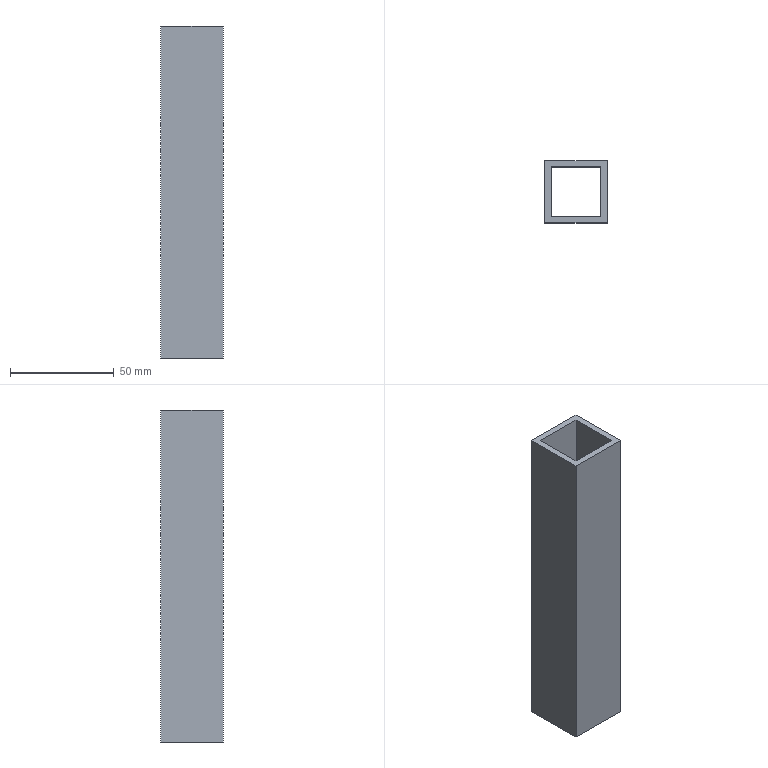Part | SolidWorks | features Extrusion 1 | 1 solid | 10 faces | box 30 x 30 x 160 mm | volume 51840 mm3 | plane 10
STEP:
#1=CARTESIAN_POINT('',(-15.,15.,80.));
#2=VERTEX_POINT('',#1);
#3=CARTESIAN_POINT('',(-15.,-15.,80.));
#4=VERTEX_POINT('',#3);
#5=CARTESIAN_POINT('',(-15.,15.,80.));
#6=DIRECTION('',(0.,-1.,0.));
#7=VECTOR('',#6,1000.);
#8=LINE('',#5,#7);
#9=EDGE_CURVE('',#2,#4,#8,.T.);
#10=ORIENTED_EDGE('',*,*,#9,.F.);
#11=CARTESIAN_POINT('',(-15.,15.,-80.));
#12=VERTEX_POINT('',#11);
#13=CARTESIAN_POINT('',(-15.,15.,-80.));
#14=DIRECTION('',(0.,0.,1.));
#15=VECTOR('',#14,1000.);
#16=LINE('',#13,#15);
#17=EDGE_CURVE('',#12,#2,#16,.T.);
#18=ORIENTED_EDGE('',*,*,#17,.F.);
#19=CARTESIAN_POINT('',(-15.,-15.,-80.));
#20=VERTEX_POINT('',#19);
#21=CARTESIAN_POINT('',(-15.,15.,-80.));
#22=DIRECTION('',(0.,-1.,0.));
#23=VECTOR('',#22,1000.);
#24=LINE('',#21,#23);
#25=EDGE_CURVE('',#12,#20,#24,.T.);
#26=ORIENTED_EDGE('',*,*,#25,.T.);
#27=CARTESIAN_POINT('',(-15.,-15.,-80.));
#28=DIRECTION('',(0.,0.,1.));
#29=VECTOR('',#28,1000.);
#30=LINE('',#27,#29);
#31=EDGE_CURVE('',#20,#4,#30,.T.);
#32=ORIENTED_EDGE('',*,*,#31,.T.);
#33=EDGE_LOOP('',(#10,#18,#26,#32));
#34=FACE_OUTER_BOUND('',#33,.T.);
#35=CARTESIAN_POINT('',(-15.,15.,-80.));
#36=DIRECTION('',(-1.,0.,0.));
#37=DIRECTION('',(0.,0.,1.));
#38=AXIS2_PLACEMENT_3D('',#35,#36,#37);
#39=PLANE('',#38);
#40=ADVANCED_FACE('',(#34),#39,.T.);
#41=CARTESIAN_POINT('',(15.,15.,80.));
#42=VERTEX_POINT('',#41);
#43=CARTESIAN_POINT('',(15.,15.,80.));
#44=DIRECTION('',(-1.,0.,0.));
#45=VECTOR('',#44,1000.);
#46=LINE('',#43,#45);
#47=EDGE_CURVE('',#42,#2,#46,.T.);
#48=ORIENTED_EDGE('',*,*,#47,.F.);
#49=CARTESIAN_POINT('',(15.,15.,-80.));
#50=VERTEX_POINT('',#49);
#51=CARTESIAN_POINT('',(15.,15.,-80.));
#52=DIRECTION('',(0.,0.,1.));
#53=VECTOR('',#52,1000.);
#54=LINE('',#51,#53);
#55=EDGE_CURVE('',#50,#42,#54,.T.);
#56=ORIENTED_EDGE('',*,*,#55,.F.);
#57=CARTESIAN_POINT('',(15.,15.,-80.));
#58=DIRECTION('',(-1.,0.,0.));
#59=VECTOR('',#58,1000.);
#60=LINE('',#57,#59);
#61=EDGE_CURVE('',#50,#12,#60,.T.);
#62=ORIENTED_EDGE('',*,*,#61,.T.);
#63=ORIENTED_EDGE('',*,*,#17,.T.);
#64=EDGE_LOOP('',(#48,#56,#62,#63));
#65=FACE_OUTER_BOUND('',#64,.T.);
#66=CARTESIAN_POINT('',(15.,15.,-80.));
#67=DIRECTION('',(0.,1.,0.));
#68=DIRECTION('',(0.,0.,1.));
#69=AXIS2_PLACEMENT_3D('',#66,#67,#68);
#70=PLANE('',#69);
#71=ADVANCED_FACE('',(#65),#70,.T.);
#72=CARTESIAN_POINT('',(15.,-15.,80.));
#73=VERTEX_POINT('',#72);
#74=CARTESIAN_POINT('',(15.,-15.,80.));
#75=DIRECTION('',(0.,1.,0.));
#76=VECTOR('',#75,1000.);
#77=LINE('',#74,#76);
#78=EDGE_CURVE('',#73,#42,#77,.T.);
#79=ORIENTED_EDGE('',*,*,#78,.F.);
#80=CARTESIAN_POINT('',(15.,-15.,-80.));
#81=VERTEX_POINT('',#80);
#82=CARTESIAN_POINT('',(15.,-15.,-80.));
#83=DIRECTION('',(0.,0.,1.));
#84=VECTOR('',#83,1000.);
#85=LINE('',#82,#84);
#86=EDGE_CURVE('',#81,#73,#85,.T.);
#87=ORIENTED_EDGE('',*,*,#86,.F.);
#88=CARTESIAN_POINT('',(15.,-15.,-80.));
#89=DIRECTION('',(0.,1.,0.));
#90=VECTOR('',#89,1000.);
#91=LINE('',#88,#90);
#92=EDGE_CURVE('',#81,#50,#91,.T.);
#93=ORIENTED_EDGE('',*,*,#92,.T.);
#94=ORIENTED_EDGE('',*,*,#55,.T.);
#95=EDGE_LOOP('',(#79,#87,#93,#94));
#96=FACE_OUTER_BOUND('',#95,.T.);
#97=CARTESIAN_POINT('',(15.,-15.,-80.));
#98=DIRECTION('',(1.,0.,0.));
#99=DIRECTION('',(0.,0.,-1.));
#100=AXIS2_PLACEMENT_3D('',#97,#98,#99);
#101=PLANE('',#100);
#102=ADVANCED_FACE('',(#96),#101,.T.);
#103=CARTESIAN_POINT('',(-15.,-15.,80.));
#104=DIRECTION('',(1.,0.,0.));
#105=VECTOR('',#104,1000.);
#106=LINE('',#103,#105);
#107=EDGE_CURVE('',#4,#73,#106,.T.);
#108=ORIENTED_EDGE('',*,*,#107,.F.);
#109=ORIENTED_EDGE('',*,*,#31,.F.);
#110=CARTESIAN_POINT('',(-15.,-15.,-80.));
#111=DIRECTION('',(1.,0.,0.));
#112=VECTOR('',#111,1000.);
#113=LINE('',#110,#112);
#114=EDGE_CURVE('',#20,#81,#113,.T.);
#115=ORIENTED_EDGE('',*,*,#114,.T.);
#116=ORIENTED_EDGE('',*,*,#86,.T.);
#117=EDGE_LOOP('',(#108,#109,#115,#116));
#118=FACE_OUTER_BOUND('',#117,.T.);
#119=CARTESIAN_POINT('',(-15.,-15.,-80.));
#120=DIRECTION('',(0.,-1.,0.));
#121=DIRECTION('',(0.,0.,-1.));
#122=AXIS2_PLACEMENT_3D('',#119,#120,#121);
#123=PLANE('',#122);
#124=ADVANCED_FACE('',(#118),#123,.T.);
#125=CARTESIAN_POINT('',(12.,12.,-80.));
#126=VERTEX_POINT('',#125);
#127=CARTESIAN_POINT('',(-12.,12.,-80.));
#128=VERTEX_POINT('',#127);
#129=CARTESIAN_POINT('',(12.,12.,-80.));
#130=DIRECTION('',(-1.,0.,0.));
#131=VECTOR('',#130,1000.);
#132=LINE('',#129,#131);
#133=EDGE_CURVE('',#126,#128,#132,.T.);
#134=ORIENTED_EDGE('',*,*,#133,.T.);
#135=CARTESIAN_POINT('',(-12.,-12.,-80.));
#136=VERTEX_POINT('',#135);
#137=CARTESIAN_POINT('',(-12.,12.,-80.));
#138=DIRECTION('',(0.,-1.,0.));
#139=VECTOR('',#138,1000.);
#140=LINE('',#137,#139);
#141=EDGE_CURVE('',#128,#136,#140,.T.);
#142=ORIENTED_EDGE('',*,*,#141,.T.);
#143=CARTESIAN_POINT('',(12.,-12.,-80.));
#144=VERTEX_POINT('',#143);
#145=CARTESIAN_POINT('',(-12.,-12.,-80.));
#146=DIRECTION('',(1.,0.,0.));
#147=VECTOR('',#146,1000.);
#148=LINE('',#145,#147);
#149=EDGE_CURVE('',#136,#144,#148,.T.);
#150=ORIENTED_EDGE('',*,*,#149,.T.);
#151=CARTESIAN_POINT('',(12.,-12.,-80.));
#152=DIRECTION('',(0.,1.,0.));
#153=VECTOR('',#152,1000.);
#154=LINE('',#151,#153);
#155=EDGE_CURVE('',#144,#126,#154,.T.);
#156=ORIENTED_EDGE('',*,*,#155,.T.);
#157=EDGE_LOOP('',(#134,#142,#150,#156));
#158=FACE_BOUND('',#157,.T.);
#159=ORIENTED_EDGE('',*,*,#25,.F.);
#160=ORIENTED_EDGE('',*,*,#61,.F.);
#161=ORIENTED_EDGE('',*,*,#92,.F.);
#162=ORIENTED_EDGE('',*,*,#114,.F.);
#163=EDGE_LOOP('',(#159,#160,#161,#162));
#164=FACE_OUTER_BOUND('',#163,.T.);
#165=CARTESIAN_POINT('',(0.,0.,-80.));
#166=DIRECTION('',(0.,0.,1.));
#167=DIRECTION('',(1.,0.,0.));
#168=AXIS2_PLACEMENT_3D('',#165,#166,#167);
#169=PLANE('',#168);
#170=ADVANCED_FACE('',(#158,#164),#169,.F.);
#171=CARTESIAN_POINT('',(-12.,12.,80.));
#172=VERTEX_POINT('',#171);
#173=CARTESIAN_POINT('',(-12.,-12.,80.));
#174=VERTEX_POINT('',#173);
#175=CARTESIAN_POINT('',(-12.,12.,80.));
#176=DIRECTION('',(0.,-1.,0.));
#177=VECTOR('',#176,1000.);
#178=LINE('',#175,#177);
#179=EDGE_CURVE('',#172,#174,#178,.T.);
#180=ORIENTED_EDGE('',*,*,#179,.F.);
#181=CARTESIAN_POINT('',(12.,12.,80.));
#182=VERTEX_POINT('',#181);
#183=CARTESIAN_POINT('',(12.,12.,80.));
#184=DIRECTION('',(-1.,0.,0.));
#185=VECTOR('',#184,1000.);
#186=LINE('',#183,#185);
#187=EDGE_CURVE('',#182,#172,#186,.T.);
#188=ORIENTED_EDGE('',*,*,#187,.F.);
#189=CARTESIAN_POINT('',(12.,-12.,80.));
#190=VERTEX_POINT('',#189);
#191=CARTESIAN_POINT('',(12.,-12.,80.));
#192=DIRECTION('',(0.,1.,0.));
#193=VECTOR('',#192,1000.);
#194=LINE('',#191,#193);
#195=EDGE_CURVE('',#190,#182,#194,.T.);
#196=ORIENTED_EDGE('',*,*,#195,.F.);
#197=CARTESIAN_POINT('',(-12.,-12.,80.));
#198=DIRECTION('',(1.,0.,0.));
#199=VECTOR('',#198,1000.);
#200=LINE('',#197,#199);
#201=EDGE_CURVE('',#174,#190,#200,.T.);
#202=ORIENTED_EDGE('',*,*,#201,.F.);
#203=EDGE_LOOP('',(#180,#188,#196,#202));
#204=FACE_BOUND('',#203,.T.);
#205=ORIENTED_EDGE('',*,*,#9,.T.);
#206=ORIENTED_EDGE('',*,*,#107,.T.);
#207=ORIENTED_EDGE('',*,*,#78,.T.);
#208=ORIENTED_EDGE('',*,*,#47,.T.);
#209=EDGE_LOOP('',(#205,#206,#207,#208));
#210=FACE_OUTER_BOUND('',#209,.T.);
#211=CARTESIAN_POINT('',(0.,0.,80.));
#212=DIRECTION('',(0.,0.,1.));
#213=DIRECTION('',(1.,0.,0.));
#214=AXIS2_PLACEMENT_3D('',#211,#212,#213);
#215=PLANE('',#214);
#216=ADVANCED_FACE('',(#204,#210),#215,.T.);
#217=ORIENTED_EDGE('',*,*,#179,.T.);
#218=CARTESIAN_POINT('',(-12.,-12.,-80.));
#219=DIRECTION('',(0.,0.,1.));
#220=VECTOR('',#219,1000.);
#221=LINE('',#218,#220);
#222=EDGE_CURVE('',#136,#174,#221,.T.);
#223=ORIENTED_EDGE('',*,*,#222,.F.);
#224=ORIENTED_EDGE('',*,*,#141,.F.);
#225=CARTESIAN_POINT('',(-12.,12.,-80.));
#226=DIRECTION('',(0.,0.,1.));
#227=VECTOR('',#226,1000.);
#228=LINE('',#225,#227);
#229=EDGE_CURVE('',#128,#172,#228,.T.);
#230=ORIENTED_EDGE('',*,*,#229,.T.);
#231=EDGE_LOOP('',(#217,#223,#224,#230));
#232=FACE_OUTER_BOUND('',#231,.T.);
#233=CARTESIAN_POINT('',(-12.,12.,-80.));
#234=DIRECTION('',(-1.,0.,0.));
#235=DIRECTION('',(0.,0.,1.));
#236=AXIS2_PLACEMENT_3D('',#233,#234,#235);
#237=PLANE('',#236);
#238=ADVANCED_FACE('',(#232),#237,.F.);
#239=ORIENTED_EDGE('',*,*,#187,.T.);
#240=ORIENTED_EDGE('',*,*,#229,.F.);
#241=ORIENTED_EDGE('',*,*,#133,.F.);
#242=CARTESIAN_POINT('',(12.,12.,-80.));
#243=DIRECTION('',(0.,0.,1.));
#244=VECTOR('',#243,1000.);
#245=LINE('',#242,#244);
#246=EDGE_CURVE('',#126,#182,#245,.T.);
#247=ORIENTED_EDGE('',*,*,#246,.T.);
#248=EDGE_LOOP('',(#239,#240,#241,#247));
#249=FACE_OUTER_BOUND('',#248,.T.);
#250=CARTESIAN_POINT('',(12.,12.,-80.));
#251=DIRECTION('',(0.,1.,0.));
#252=DIRECTION('',(0.,0.,1.));
#253=AXIS2_PLACEMENT_3D('',#250,#251,#252);
#254=PLANE('',#253);
#255=ADVANCED_FACE('',(#249),#254,.F.);
#256=ORIENTED_EDGE('',*,*,#195,.T.);
#257=ORIENTED_EDGE('',*,*,#246,.F.);
#258=ORIENTED_EDGE('',*,*,#155,.F.);
#259=CARTESIAN_POINT('',(12.,-12.,-80.));
#260=DIRECTION('',(0.,0.,1.));
#261=VECTOR('',#260,1000.);
#262=LINE('',#259,#261);
#263=EDGE_CURVE('',#144,#190,#262,.T.);
#264=ORIENTED_EDGE('',*,*,#263,.T.);
#265=EDGE_LOOP('',(#256,#257,#258,#264));
#266=FACE_OUTER_BOUND('',#265,.T.);
#267=CARTESIAN_POINT('',(12.,-12.,-80.));
#268=DIRECTION('',(1.,0.,0.));
#269=DIRECTION('',(0.,0.,-1.));
#270=AXIS2_PLACEMENT_3D('',#267,#268,#269);
#271=PLANE('',#270);
#272=ADVANCED_FACE('',(#266),#271,.F.);
#273=ORIENTED_EDGE('',*,*,#201,.T.);
#274=ORIENTED_EDGE('',*,*,#263,.F.);
#275=ORIENTED_EDGE('',*,*,#149,.F.);
#276=ORIENTED_EDGE('',*,*,#222,.T.);
#277=EDGE_LOOP('',(#273,#274,#275,#276));
#278=FACE_OUTER_BOUND('',#277,.T.);
#279=CARTESIAN_POINT('',(-12.,-12.,-80.));
#280=DIRECTION('',(0.,-1.,0.));
#281=DIRECTION('',(0.,0.,-1.));
#282=AXIS2_PLACEMENT_3D('',#279,#280,#281);
#283=PLANE('',#282);
#284=ADVANCED_FACE('',(#278),#283,.F.);
#285=CLOSED_SHELL('',(#40,#71,#102,#124,#170,#216,#238,#255,#272,#284));
#286=MANIFOLD_SOLID_BREP('',#285);
#287=CARTESIAN_POINT('',(0.,0.,0.));
#288=DIRECTION('',(0.,0.,1.));
#289=DIRECTION('',(1.,0.,0.));
#290=AXIS2_PLACEMENT_3D('',#287,#288,#289);
#291=(LENGTH_UNIT()NAMED_UNIT(*)SI_UNIT(.MILLI.,.METRE.));
#292=UNCERTAINTY_MEASURE_WITH_UNIT(LENGTH_MEASURE(0.00001),#291,'','');
#293=(NAMED_UNIT(*)PLANE_ANGLE_UNIT()SI_UNIT($,.RADIAN.));
#294=(NAMED_UNIT(*)SI_UNIT($,.STERADIAN.)SOLID_ANGLE_UNIT());
#295=(GEOMETRIC_REPRESENTATION_CONTEXT(3)GLOBAL_UNCERTAINTY_ASSIGNED_CONTEXT((#292))GLOBAL_UNIT_ASSIGNED_CONTEXT((#291,#293,#294))REPRESENTATION_CONTEXT('',''));
#296=ADVANCED_BREP_SHAPE_REPRESENTATION('',(#286,#290),#295);